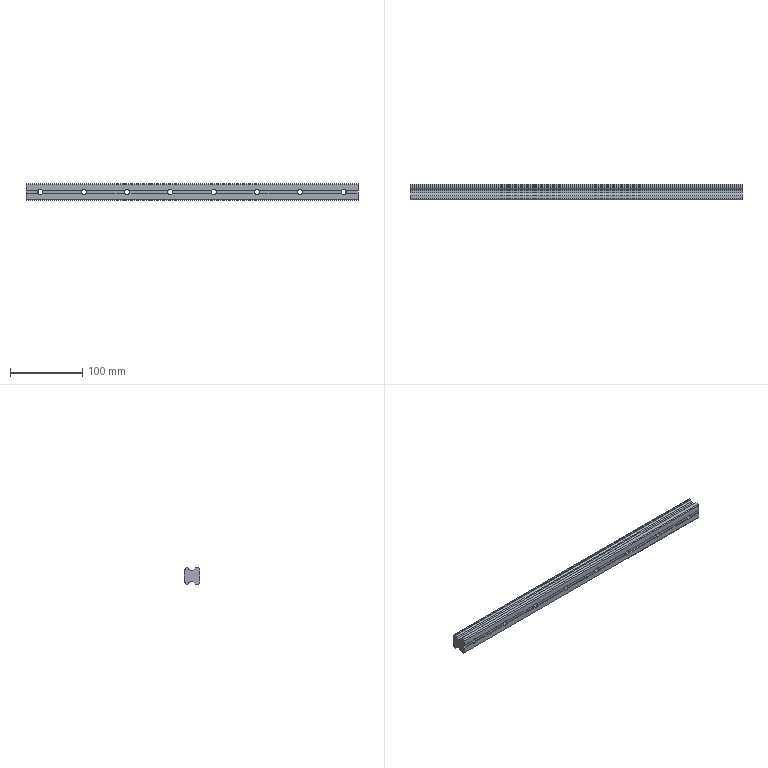Part | SolidWorks | features BaseBody 1 | 1 solid | 94 faces | box 460 x 22 x 23 mm | volume 189188 mm3 | plane 58 | cylinder 36 | commonest cylinder face diameters 7 x16 11 x16 4.96 x4